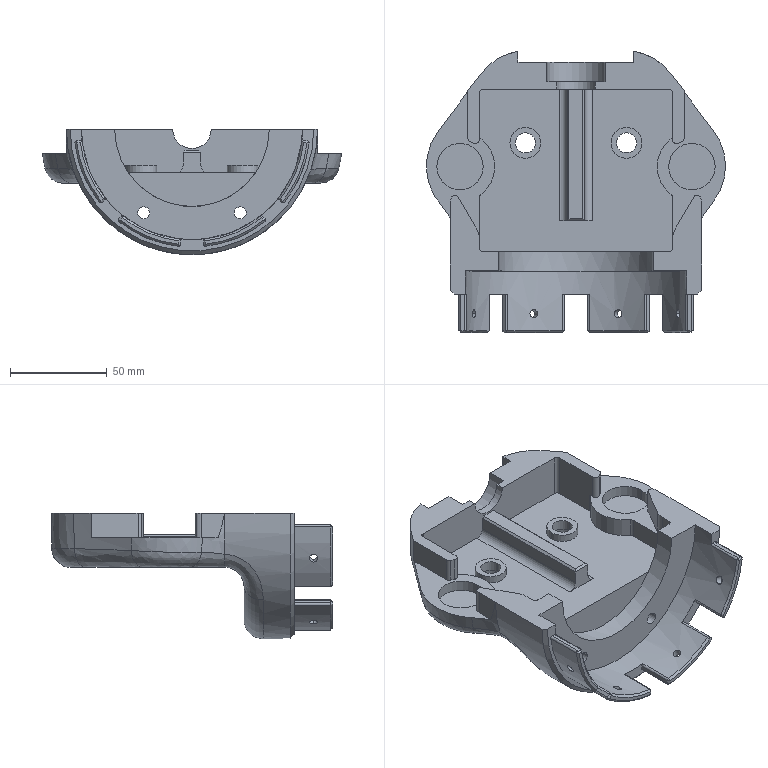Part | NX | features BREP 1 | 1 solid | 206 faces | box 154.814 x 145.413 x 65 mm | volume 219236 mm3 | cylinder 91 | plane 68 | cone 28 | spline 18 | torus 1 | commonest cylinder face diameters 2 x19 4 x14 4.2 x8 20 x5 6.2 x4 7.2 x4